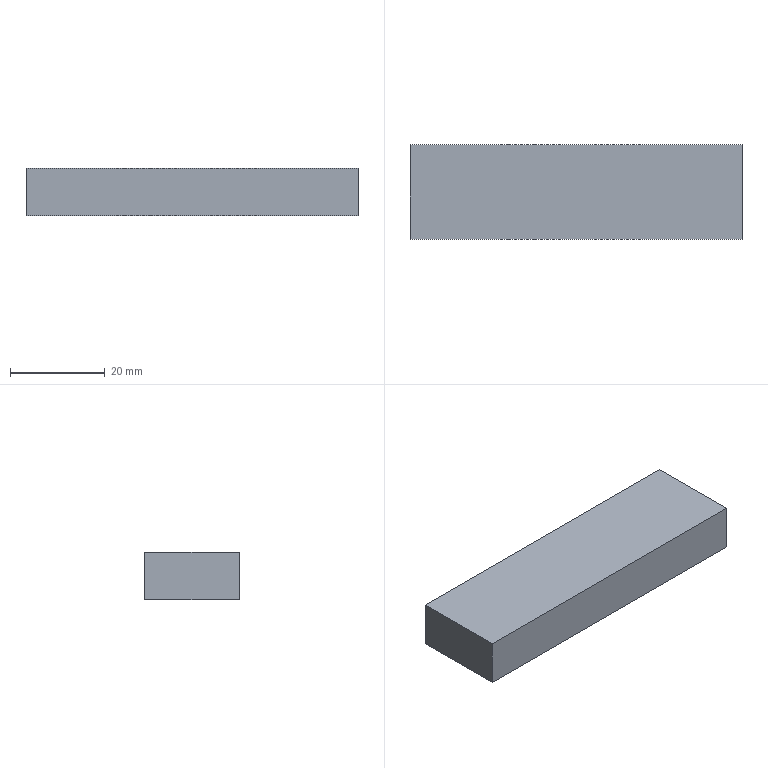Part | SolidWorks | features Extrusion 1 | 1 solid | 6 faces | box 70 x 20 x 10 mm | volume 14000 mm3 | plane 6
STEP:
#1=CARTESIAN_POINT('',(35.,-10.,0.));
#2=VERTEX_POINT('',#1);
#3=CARTESIAN_POINT('',(35.,10.,0.));
#4=VERTEX_POINT('',#3);
#5=CARTESIAN_POINT('',(35.,10.,0.));
#6=DIRECTION('',(0.,1.,0.));
#7=VECTOR('',#6,1000.);
#8=LINE('',#5,#7);
#9=EDGE_CURVE('',#2,#4,#8,.T.);
#10=ORIENTED_EDGE('',*,*,#9,.F.);
#11=CARTESIAN_POINT('',(35.,-10.,-10.));
#12=VERTEX_POINT('',#11);
#13=CARTESIAN_POINT('',(35.,-10.,-10.));
#14=DIRECTION('',(0.,0.,1.));
#15=VECTOR('',#14,1000.);
#16=LINE('',#13,#15);
#17=EDGE_CURVE('',#12,#2,#16,.T.);
#18=ORIENTED_EDGE('',*,*,#17,.F.);
#19=CARTESIAN_POINT('',(35.,10.,-10.));
#20=VERTEX_POINT('',#19);
#21=CARTESIAN_POINT('',(35.,10.,-10.));
#22=DIRECTION('',(0.,1.,0.));
#23=VECTOR('',#22,1000.);
#24=LINE('',#21,#23);
#25=EDGE_CURVE('',#12,#20,#24,.T.);
#26=ORIENTED_EDGE('',*,*,#25,.T.);
#27=CARTESIAN_POINT('',(35.,10.,-10.));
#28=DIRECTION('',(0.,0.,1.));
#29=VECTOR('',#28,1000.);
#30=LINE('',#27,#29);
#31=EDGE_CURVE('',#20,#4,#30,.T.);
#32=ORIENTED_EDGE('',*,*,#31,.T.);
#33=EDGE_LOOP('',(#10,#18,#26,#32));
#34=FACE_OUTER_BOUND('',#33,.T.);
#35=CARTESIAN_POINT('',(35.,10.,-10.));
#36=DIRECTION('',(1.,0.,0.));
#37=DIRECTION('',(0.,1.,0.));
#38=AXIS2_PLACEMENT_3D('',#35,#36,#37);
#39=PLANE('',#38);
#40=ADVANCED_FACE('',(#34),#39,.T.);
#41=CARTESIAN_POINT('',(-35.,-10.,0.));
#42=VERTEX_POINT('',#41);
#43=CARTESIAN_POINT('',(-35.,-10.,0.));
#44=DIRECTION('',(1.,0.,0.));
#45=VECTOR('',#44,1000.);
#46=LINE('',#43,#45);
#47=EDGE_CURVE('',#42,#2,#46,.T.);
#48=ORIENTED_EDGE('',*,*,#47,.F.);
#49=CARTESIAN_POINT('',(-35.,-10.,-10.));
#50=VERTEX_POINT('',#49);
#51=CARTESIAN_POINT('',(-35.,-10.,-10.));
#52=DIRECTION('',(0.,0.,1.));
#53=VECTOR('',#52,1000.);
#54=LINE('',#51,#53);
#55=EDGE_CURVE('',#50,#42,#54,.T.);
#56=ORIENTED_EDGE('',*,*,#55,.F.);
#57=CARTESIAN_POINT('',(-35.,-10.,-10.));
#58=DIRECTION('',(1.,0.,0.));
#59=VECTOR('',#58,1000.);
#60=LINE('',#57,#59);
#61=EDGE_CURVE('',#50,#12,#60,.T.);
#62=ORIENTED_EDGE('',*,*,#61,.T.);
#63=ORIENTED_EDGE('',*,*,#17,.T.);
#64=EDGE_LOOP('',(#48,#56,#62,#63));
#65=FACE_OUTER_BOUND('',#64,.T.);
#66=CARTESIAN_POINT('',(-35.,-10.,-10.));
#67=DIRECTION('',(0.,-1.,0.));
#68=DIRECTION('',(0.,0.,-1.));
#69=AXIS2_PLACEMENT_3D('',#66,#67,#68);
#70=PLANE('',#69);
#71=ADVANCED_FACE('',(#65),#70,.T.);
#72=CARTESIAN_POINT('',(-35.,10.,0.));
#73=VERTEX_POINT('',#72);
#74=CARTESIAN_POINT('',(-35.,10.,0.));
#75=DIRECTION('',(0.,-1.,0.));
#76=VECTOR('',#75,1000.);
#77=LINE('',#74,#76);
#78=EDGE_CURVE('',#73,#42,#77,.T.);
#79=ORIENTED_EDGE('',*,*,#78,.F.);
#80=CARTESIAN_POINT('',(-35.,10.,-10.));
#81=VERTEX_POINT('',#80);
#82=CARTESIAN_POINT('',(-35.,10.,-10.));
#83=DIRECTION('',(0.,0.,1.));
#84=VECTOR('',#83,1000.);
#85=LINE('',#82,#84);
#86=EDGE_CURVE('',#81,#73,#85,.T.);
#87=ORIENTED_EDGE('',*,*,#86,.F.);
#88=CARTESIAN_POINT('',(-35.,10.,-10.));
#89=DIRECTION('',(0.,-1.,0.));
#90=VECTOR('',#89,1000.);
#91=LINE('',#88,#90);
#92=EDGE_CURVE('',#81,#50,#91,.T.);
#93=ORIENTED_EDGE('',*,*,#92,.T.);
#94=ORIENTED_EDGE('',*,*,#55,.T.);
#95=EDGE_LOOP('',(#79,#87,#93,#94));
#96=FACE_OUTER_BOUND('',#95,.T.);
#97=CARTESIAN_POINT('',(-35.,10.,-10.));
#98=DIRECTION('',(-1.,0.,0.));
#99=DIRECTION('',(0.,0.,1.));
#100=AXIS2_PLACEMENT_3D('',#97,#98,#99);
#101=PLANE('',#100);
#102=ADVANCED_FACE('',(#96),#101,.T.);
#103=CARTESIAN_POINT('',(-35.,10.,0.));
#104=DIRECTION('',(-1.,0.,0.));
#105=VECTOR('',#104,1000.);
#106=LINE('',#103,#105);
#107=EDGE_CURVE('',#4,#73,#106,.T.);
#108=ORIENTED_EDGE('',*,*,#107,.F.);
#109=ORIENTED_EDGE('',*,*,#31,.F.);
#110=CARTESIAN_POINT('',(-35.,10.,-10.));
#111=DIRECTION('',(-1.,0.,0.));
#112=VECTOR('',#111,1000.);
#113=LINE('',#110,#112);
#114=EDGE_CURVE('',#20,#81,#113,.T.);
#115=ORIENTED_EDGE('',*,*,#114,.T.);
#116=ORIENTED_EDGE('',*,*,#86,.T.);
#117=EDGE_LOOP('',(#108,#109,#115,#116));
#118=FACE_OUTER_BOUND('',#117,.T.);
#119=CARTESIAN_POINT('',(-35.,10.,-10.));
#120=DIRECTION('',(0.,1.,0.));
#121=DIRECTION('',(0.,0.,1.));
#122=AXIS2_PLACEMENT_3D('',#119,#120,#121);
#123=PLANE('',#122);
#124=ADVANCED_FACE('',(#118),#123,.T.);
#125=ORIENTED_EDGE('',*,*,#25,.F.);
#126=ORIENTED_EDGE('',*,*,#61,.F.);
#127=ORIENTED_EDGE('',*,*,#92,.F.);
#128=ORIENTED_EDGE('',*,*,#114,.F.);
#129=EDGE_LOOP('',(#125,#126,#127,#128));
#130=FACE_OUTER_BOUND('',#129,.T.);
#131=CARTESIAN_POINT('',(0.,0.,-10.));
#132=DIRECTION('',(0.,0.,1.));
#133=DIRECTION('',(1.,0.,0.));
#134=AXIS2_PLACEMENT_3D('',#131,#132,#133);
#135=PLANE('',#134);
#136=ADVANCED_FACE('',(#130),#135,.F.);
#137=ORIENTED_EDGE('',*,*,#9,.T.);
#138=ORIENTED_EDGE('',*,*,#107,.T.);
#139=ORIENTED_EDGE('',*,*,#78,.T.);
#140=ORIENTED_EDGE('',*,*,#47,.T.);
#141=EDGE_LOOP('',(#137,#138,#139,#140));
#142=FACE_OUTER_BOUND('',#141,.T.);
#143=CARTESIAN_POINT('',(0.,0.,0.));
#144=DIRECTION('',(0.,0.,1.));
#145=DIRECTION('',(1.,0.,0.));
#146=AXIS2_PLACEMENT_3D('',#143,#144,#145);
#147=PLANE('',#146);
#148=ADVANCED_FACE('',(#142),#147,.T.);
#149=CLOSED_SHELL('',(#40,#71,#102,#124,#136,#148));
#150=MANIFOLD_SOLID_BREP('',#149);
#151=CARTESIAN_POINT('',(0.,0.,0.));
#152=DIRECTION('',(0.,0.,1.));
#153=DIRECTION('',(1.,0.,0.));
#154=AXIS2_PLACEMENT_3D('',#151,#152,#153);
#155=(LENGTH_UNIT()NAMED_UNIT(*)SI_UNIT(.MILLI.,.METRE.));
#156=UNCERTAINTY_MEASURE_WITH_UNIT(LENGTH_MEASURE(0.00001),#155,'','');
#157=(NAMED_UNIT(*)PLANE_ANGLE_UNIT()SI_UNIT($,.RADIAN.));
#158=(NAMED_UNIT(*)SI_UNIT($,.STERADIAN.)SOLID_ANGLE_UNIT());
#159=(GEOMETRIC_REPRESENTATION_CONTEXT(3)GLOBAL_UNCERTAINTY_ASSIGNED_CONTEXT((#156))GLOBAL_UNIT_ASSIGNED_CONTEXT((#155,#157,#158))REPRESENTATION_CONTEXT('',''));
#160=ADVANCED_BREP_SHAPE_REPRESENTATION('',(#150,#154),#159);